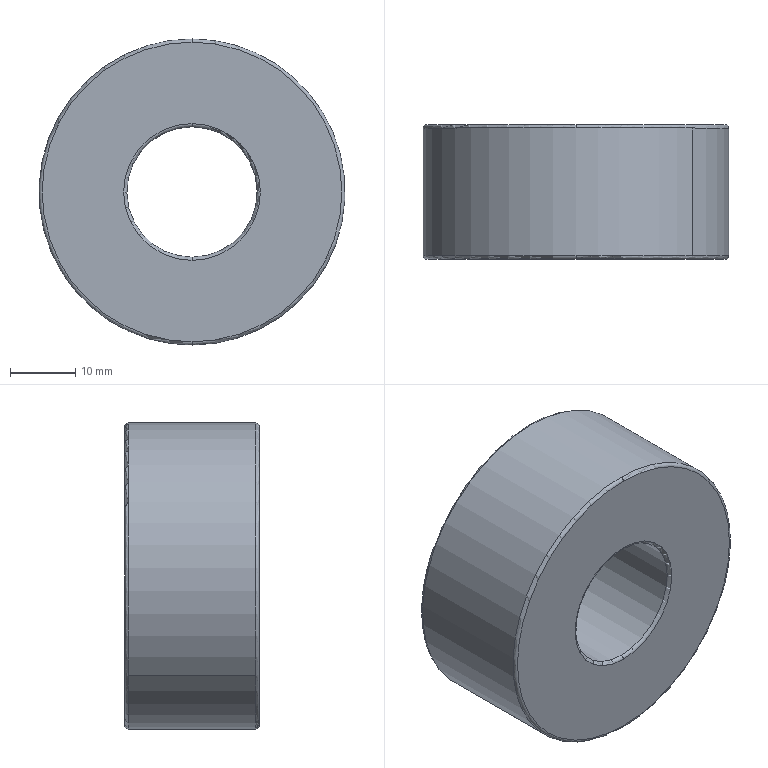Part | SolidWorks | features BaseBody 1 | 1 solid | 14 faces | box 47 x 20.6 x 47 mm | volume 29246 mm3 | torus 8 | cylinder 4 | plane 2 | commonest cylinder face diameters 20 x2 47 x2
STEP:
#1=CARTESIAN_POINT('',(624.451,36.7,7.283));
#2=VERTEX_POINT('',#1);
#3=CARTESIAN_POINT('',(624.451,36.7,28.283));
#4=VERTEX_POINT('',#3);
#5=CARTESIAN_POINT('',(624.451,36.7,17.783));
#6=DIRECTION('',(0.,1.,0.));
#7=DIRECTION('',(0.,0.,-1.));
#8=AXIS2_PLACEMENT_3D('',#5,#6,#7);
#9=CIRCLE('',#8,10.5);
#10=EDGE_CURVE('',#2,#4,#9,.T.);
#11=ORIENTED_EDGE('',*,*,#10,.F.);
#12=CARTESIAN_POINT('',(624.451,37.2,7.783));
#13=VERTEX_POINT('',#12);
#14=CARTESIAN_POINT('',(624.451,37.2,7.283));
#15=DIRECTION('',(-1.,0.,0.));
#16=DIRECTION('',(0.,0.,1.));
#17=AXIS2_PLACEMENT_3D('',#14,#15,#16);
#18=CIRCLE('',#17,0.5);
#19=EDGE_CURVE('',#2,#13,#18,.T.);
#20=ORIENTED_EDGE('',*,*,#19,.T.);
#21=CARTESIAN_POINT('',(616.859,37.2,11.275));
#22=VERTEX_POINT('',#21);
#23=CARTESIAN_POINT('',(624.451,37.2,17.783));
#24=DIRECTION('',(0.,1.,0.));
#25=DIRECTION('',(0.,0.,-1.));
#26=AXIS2_PLACEMENT_3D('',#23,#24,#25);
#27=CIRCLE('',#26,10.);
#28=EDGE_CURVE('',#13,#22,#27,.T.);
#29=ORIENTED_EDGE('',*,*,#28,.T.);
#30=CARTESIAN_POINT('',(624.451,37.2,27.783));
#31=VERTEX_POINT('',#30);
#32=CARTESIAN_POINT('',(624.451,37.2,17.783));
#33=DIRECTION('',(0.,1.,0.));
#34=DIRECTION('',(0.,0.,-1.));
#35=AXIS2_PLACEMENT_3D('',#32,#33,#34);
#36=CIRCLE('',#35,10.);
#37=EDGE_CURVE('',#22,#31,#36,.T.);
#38=ORIENTED_EDGE('',*,*,#37,.T.);
#39=CARTESIAN_POINT('',(624.451,37.2,28.283));
#40=DIRECTION('',(1.,0.,0.));
#41=DIRECTION('',(0.,0.,-1.));
#42=AXIS2_PLACEMENT_3D('',#39,#40,#41);
#43=CIRCLE('',#42,0.5);
#44=EDGE_CURVE('',#4,#31,#43,.T.);
#45=ORIENTED_EDGE('',*,*,#44,.F.);
#46=EDGE_LOOP('',(#11,#20,#29,#38,#45));
#47=FACE_OUTER_BOUND('',#46,.T.);
#48=CARTESIAN_POINT('',(624.451,37.2,17.783));
#49=DIRECTION('',(0.,-1.,0.));
#50=DIRECTION('',(0.,0.,1.));
#51=AXIS2_PLACEMENT_3D('',#48,#49,#50);
#52=TOROIDAL_SURFACE('',#51,10.5,0.5);
#53=ADVANCED_FACE('',(#47),#52,.T.);
#54=CARTESIAN_POINT('',(606.61,37.2,2.488));
#55=VERTEX_POINT('',#54);
#56=CARTESIAN_POINT('',(624.451,37.2,-5.717));
#57=VERTEX_POINT('',#56);
#58=CARTESIAN_POINT('',(624.451,37.2,17.783));
#59=DIRECTION('',(0.,-1.,0.));
#60=DIRECTION('',(0.,0.,-1.));
#61=AXIS2_PLACEMENT_3D('',#58,#59,#60);
#62=CIRCLE('',#61,23.5);
#63=EDGE_CURVE('',#55,#57,#62,.T.);
#64=ORIENTED_EDGE('',*,*,#63,.T.);
#65=CARTESIAN_POINT('',(624.451,36.7,-5.217));
#66=VERTEX_POINT('',#65);
#67=CARTESIAN_POINT('',(624.451,37.2,-5.217));
#68=DIRECTION('',(-1.,0.,0.));
#69=DIRECTION('',(0.,0.,1.));
#70=AXIS2_PLACEMENT_3D('',#67,#68,#69);
#71=CIRCLE('',#70,0.5);
#72=EDGE_CURVE('',#57,#66,#71,.T.);
#73=ORIENTED_EDGE('',*,*,#72,.T.);
#74=CARTESIAN_POINT('',(624.451,36.7,40.783));
#75=VERTEX_POINT('',#74);
#76=CARTESIAN_POINT('',(624.451,36.7,17.783));
#77=DIRECTION('',(0.,-1.,0.));
#78=DIRECTION('',(0.,0.,-1.));
#79=AXIS2_PLACEMENT_3D('',#76,#77,#78);
#80=CIRCLE('',#79,23.);
#81=EDGE_CURVE('',#75,#66,#80,.T.);
#82=ORIENTED_EDGE('',*,*,#81,.F.);
#83=CARTESIAN_POINT('',(624.451,37.2,41.283));
#84=VERTEX_POINT('',#83);
#85=CARTESIAN_POINT('',(624.451,37.2,40.783));
#86=DIRECTION('',(1.,0.,0.));
#87=DIRECTION('',(0.,0.,-1.));
#88=AXIS2_PLACEMENT_3D('',#85,#86,#87);
#89=CIRCLE('',#88,0.5);
#90=EDGE_CURVE('',#84,#75,#89,.T.);
#91=ORIENTED_EDGE('',*,*,#90,.F.);
#92=CARTESIAN_POINT('',(624.451,37.2,17.783));
#93=DIRECTION('',(0.,-1.,0.));
#94=DIRECTION('',(0.,0.,-1.));
#95=AXIS2_PLACEMENT_3D('',#92,#93,#94);
#96=CIRCLE('',#95,23.5);
#97=EDGE_CURVE('',#84,#55,#96,.T.);
#98=ORIENTED_EDGE('',*,*,#97,.T.);
#99=EDGE_LOOP('',(#64,#73,#82,#91,#98));
#100=FACE_OUTER_BOUND('',#99,.T.);
#101=CARTESIAN_POINT('',(624.451,37.2,17.783));
#102=DIRECTION('',(0.,-1.,0.));
#103=DIRECTION('',(0.,0.,1.));
#104=AXIS2_PLACEMENT_3D('',#101,#102,#103);
#105=TOROIDAL_SURFACE('',#104,23.,0.5);
#106=ADVANCED_FACE('',(#100),#105,.T.);
#107=CARTESIAN_POINT('',(624.451,56.8,41.283));
#108=VERTEX_POINT('',#107);
#109=CARTESIAN_POINT('',(606.61,56.8,2.488));
#110=VERTEX_POINT('',#109);
#111=CARTESIAN_POINT('',(624.451,56.8,17.783));
#112=DIRECTION('',(0.,-1.,0.));
#113=DIRECTION('',(0.,0.,1.));
#114=AXIS2_PLACEMENT_3D('',#111,#112,#113);
#115=CIRCLE('',#114,23.5);
#116=EDGE_CURVE('',#108,#110,#115,.T.);
#117=ORIENTED_EDGE('',*,*,#116,.F.);
#118=CARTESIAN_POINT('',(624.451,57.3,40.783));
#119=VERTEX_POINT('',#118);
#120=CARTESIAN_POINT('',(624.451,56.8,40.783));
#121=DIRECTION('',(-1.,0.,0.));
#122=DIRECTION('',(0.,0.,1.));
#123=AXIS2_PLACEMENT_3D('',#120,#121,#122);
#124=CIRCLE('',#123,0.5);
#125=EDGE_CURVE('',#108,#119,#124,.T.);
#126=ORIENTED_EDGE('',*,*,#125,.T.);
#127=CARTESIAN_POINT('',(624.451,57.3,-5.217));
#128=VERTEX_POINT('',#127);
#129=CARTESIAN_POINT('',(624.451,57.3,17.783));
#130=DIRECTION('',(0.,-1.,0.));
#131=DIRECTION('',(0.,0.,1.));
#132=AXIS2_PLACEMENT_3D('',#129,#130,#131);
#133=CIRCLE('',#132,23.);
#134=EDGE_CURVE('',#119,#128,#133,.T.);
#135=ORIENTED_EDGE('',*,*,#134,.T.);
#136=CARTESIAN_POINT('',(624.451,56.8,-5.717));
#137=VERTEX_POINT('',#136);
#138=CARTESIAN_POINT('',(624.451,56.8,-5.217));
#139=DIRECTION('',(1.,0.,0.));
#140=DIRECTION('',(0.,0.,-1.));
#141=AXIS2_PLACEMENT_3D('',#138,#139,#140);
#142=CIRCLE('',#141,0.5);
#143=EDGE_CURVE('',#137,#128,#142,.T.);
#144=ORIENTED_EDGE('',*,*,#143,.F.);
#145=CARTESIAN_POINT('',(624.451,56.8,17.783));
#146=DIRECTION('',(0.,-1.,0.));
#147=DIRECTION('',(0.,0.,1.));
#148=AXIS2_PLACEMENT_3D('',#145,#146,#147);
#149=CIRCLE('',#148,23.5);
#150=EDGE_CURVE('',#110,#137,#149,.T.);
#151=ORIENTED_EDGE('',*,*,#150,.F.);
#152=EDGE_LOOP('',(#117,#126,#135,#144,#151));
#153=FACE_OUTER_BOUND('',#152,.T.);
#154=CARTESIAN_POINT('',(624.451,56.8,17.783));
#155=DIRECTION('',(0.,1.,0.));
#156=DIRECTION('',(0.,0.,-1.));
#157=AXIS2_PLACEMENT_3D('',#154,#155,#156);
#158=TOROIDAL_SURFACE('',#157,23.,0.5);
#159=ADVANCED_FACE('',(#153),#158,.T.);
#160=CARTESIAN_POINT('',(624.451,57.3,7.283));
#161=VERTEX_POINT('',#160);
#162=CARTESIAN_POINT('',(624.451,57.3,28.283));
#163=VERTEX_POINT('',#162);
#164=CARTESIAN_POINT('',(624.451,57.3,17.783));
#165=DIRECTION('',(0.,1.,0.));
#166=DIRECTION('',(0.,0.,1.));
#167=AXIS2_PLACEMENT_3D('',#164,#165,#166);
#168=CIRCLE('',#167,10.5);
#169=EDGE_CURVE('',#161,#163,#168,.T.);
#170=ORIENTED_EDGE('',*,*,#169,.T.);
#171=CARTESIAN_POINT('',(624.451,56.8,27.783));
#172=VERTEX_POINT('',#171);
#173=CARTESIAN_POINT('',(624.451,56.8,28.283));
#174=DIRECTION('',(-1.,0.,0.));
#175=DIRECTION('',(0.,0.,1.));
#176=AXIS2_PLACEMENT_3D('',#173,#174,#175);
#177=CIRCLE('',#176,0.5);
#178=EDGE_CURVE('',#163,#172,#177,.T.);
#179=ORIENTED_EDGE('',*,*,#178,.T.);
#180=CARTESIAN_POINT('',(616.859,56.8,11.275));
#181=VERTEX_POINT('',#180);
#182=CARTESIAN_POINT('',(624.451,56.8,17.783));
#183=DIRECTION('',(0.,1.,0.));
#184=DIRECTION('',(0.,0.,1.));
#185=AXIS2_PLACEMENT_3D('',#182,#183,#184);
#186=CIRCLE('',#185,10.);
#187=EDGE_CURVE('',#181,#172,#186,.T.);
#188=ORIENTED_EDGE('',*,*,#187,.F.);
#189=CARTESIAN_POINT('',(624.451,56.8,7.783));
#190=VERTEX_POINT('',#189);
#191=CARTESIAN_POINT('',(624.451,56.8,17.783));
#192=DIRECTION('',(0.,1.,0.));
#193=DIRECTION('',(0.,0.,1.));
#194=AXIS2_PLACEMENT_3D('',#191,#192,#193);
#195=CIRCLE('',#194,10.);
#196=EDGE_CURVE('',#190,#181,#195,.T.);
#197=ORIENTED_EDGE('',*,*,#196,.F.);
#198=CARTESIAN_POINT('',(624.451,56.8,7.283));
#199=DIRECTION('',(1.,0.,0.));
#200=DIRECTION('',(0.,0.,-1.));
#201=AXIS2_PLACEMENT_3D('',#198,#199,#200);
#202=CIRCLE('',#201,0.5);
#203=EDGE_CURVE('',#161,#190,#202,.T.);
#204=ORIENTED_EDGE('',*,*,#203,.F.);
#205=EDGE_LOOP('',(#170,#179,#188,#197,#204));
#206=FACE_OUTER_BOUND('',#205,.T.);
#207=CARTESIAN_POINT('',(624.451,56.8,17.783));
#208=DIRECTION('',(0.,1.,0.));
#209=DIRECTION('',(0.,0.,-1.));
#210=AXIS2_PLACEMENT_3D('',#207,#208,#209);
#211=TOROIDAL_SURFACE('',#210,10.5,0.5);
#212=ADVANCED_FACE('',(#206),#211,.T.);
#213=ORIENTED_EDGE('',*,*,#187,.T.);
#214=CARTESIAN_POINT('',(632.043,56.8,24.292));
#215=VERTEX_POINT('',#214);
#216=CARTESIAN_POINT('',(624.451,56.8,17.783));
#217=DIRECTION('',(0.,1.,0.));
#218=DIRECTION('',(0.,0.,1.));
#219=AXIS2_PLACEMENT_3D('',#216,#217,#218);
#220=CIRCLE('',#219,10.);
#221=EDGE_CURVE('',#172,#215,#220,.T.);
#222=ORIENTED_EDGE('',*,*,#221,.T.);
#223=CARTESIAN_POINT('',(632.043,37.2,24.292));
#224=VERTEX_POINT('',#223);
#225=CARTESIAN_POINT('',(632.043,46.7,24.292));
#226=DIRECTION('',(0.,-1.,0.));
#227=VECTOR('',#226,1000.);
#228=LINE('',#225,#227);
#229=EDGE_CURVE('',#215,#224,#228,.T.);
#230=ORIENTED_EDGE('',*,*,#229,.T.);
#231=CARTESIAN_POINT('',(624.451,37.2,17.783));
#232=DIRECTION('',(0.,1.,0.));
#233=DIRECTION('',(0.,0.,-1.));
#234=AXIS2_PLACEMENT_3D('',#231,#232,#233);
#235=CIRCLE('',#234,10.);
#236=EDGE_CURVE('',#31,#224,#235,.T.);
#237=ORIENTED_EDGE('',*,*,#236,.F.);
#238=ORIENTED_EDGE('',*,*,#37,.F.);
#239=CARTESIAN_POINT('',(616.859,46.7,11.275));
#240=DIRECTION('',(0.,-1.,0.));
#241=VECTOR('',#240,1000.);
#242=LINE('',#239,#241);
#243=EDGE_CURVE('',#181,#22,#242,.T.);
#244=ORIENTED_EDGE('',*,*,#243,.F.);
#245=EDGE_LOOP('',(#213,#222,#230,#237,#238,#244));
#246=FACE_OUTER_BOUND('',#245,.T.);
#247=CARTESIAN_POINT('',(624.451,46.7,17.783));
#248=DIRECTION('',(0.,-1.,0.));
#249=DIRECTION('',(-0.7592,0.,-0.6509));
#250=AXIS2_PLACEMENT_3D('',#247,#248,#249);
#251=CYLINDRICAL_SURFACE('',#250,10.);
#252=ADVANCED_FACE('',(#246),#251,.F.);
#253=ORIENTED_EDGE('',*,*,#150,.T.);
#254=CARTESIAN_POINT('',(642.292,56.8,33.079));
#255=VERTEX_POINT('',#254);
#256=CARTESIAN_POINT('',(624.451,56.8,17.783));
#257=DIRECTION('',(0.,-1.,0.));
#258=DIRECTION('',(0.,0.,1.));
#259=AXIS2_PLACEMENT_3D('',#256,#257,#258);
#260=CIRCLE('',#259,23.5);
#261=EDGE_CURVE('',#137,#255,#260,.T.);
#262=ORIENTED_EDGE('',*,*,#261,.T.);
#263=CARTESIAN_POINT('',(642.292,37.2,33.079));
#264=VERTEX_POINT('',#263);
#265=CARTESIAN_POINT('',(642.292,46.7,33.079));
#266=DIRECTION('',(0.,-1.,0.));
#267=VECTOR('',#266,1000.);
#268=LINE('',#265,#267);
#269=EDGE_CURVE('',#255,#264,#268,.T.);
#270=ORIENTED_EDGE('',*,*,#269,.T.);
#271=CARTESIAN_POINT('',(624.451,37.2,17.783));
#272=DIRECTION('',(0.,-1.,0.));
#273=DIRECTION('',(0.,0.,-1.));
#274=AXIS2_PLACEMENT_3D('',#271,#272,#273);
#275=CIRCLE('',#274,23.5);
#276=EDGE_CURVE('',#57,#264,#275,.T.);
#277=ORIENTED_EDGE('',*,*,#276,.F.);
#278=ORIENTED_EDGE('',*,*,#63,.F.);
#279=CARTESIAN_POINT('',(606.61,46.7,2.488));
#280=DIRECTION('',(0.,-1.,0.));
#281=VECTOR('',#280,1000.);
#282=LINE('',#279,#281);
#283=EDGE_CURVE('',#110,#55,#282,.T.);
#284=ORIENTED_EDGE('',*,*,#283,.F.);
#285=EDGE_LOOP('',(#253,#262,#270,#277,#278,#284));
#286=FACE_OUTER_BOUND('',#285,.T.);
#287=CARTESIAN_POINT('',(624.451,46.7,17.783));
#288=DIRECTION('',(0.,-1.,0.));
#289=DIRECTION('',(-0.7592,0.,-0.6509));
#290=AXIS2_PLACEMENT_3D('',#287,#288,#289);
#291=CYLINDRICAL_SURFACE('',#290,23.5);
#292=ADVANCED_FACE('',(#286),#291,.T.);
#293=CARTESIAN_POINT('',(624.451,36.7,17.783));
#294=DIRECTION('',(0.,1.,0.));
#295=DIRECTION('',(0.,0.,-1.));
#296=AXIS2_PLACEMENT_3D('',#293,#294,#295);
#297=CIRCLE('',#296,10.5);
#298=EDGE_CURVE('',#4,#2,#297,.T.);
#299=ORIENTED_EDGE('',*,*,#298,.T.);
#300=ORIENTED_EDGE('',*,*,#10,.T.);
#301=EDGE_LOOP('',(#299,#300));
#302=FACE_BOUND('',#301,.T.);
#303=ORIENTED_EDGE('',*,*,#81,.T.);
#304=CARTESIAN_POINT('',(624.451,36.7,17.783));
#305=DIRECTION('',(0.,-1.,0.));
#306=DIRECTION('',(0.,0.,-1.));
#307=AXIS2_PLACEMENT_3D('',#304,#305,#306);
#308=CIRCLE('',#307,23.);
#309=EDGE_CURVE('',#66,#75,#308,.T.);
#310=ORIENTED_EDGE('',*,*,#309,.T.);
#311=EDGE_LOOP('',(#303,#310));
#312=FACE_OUTER_BOUND('',#311,.T.);
#313=CARTESIAN_POINT('',(624.451,36.7,17.783));
#314=DIRECTION('',(0.,-1.,0.));
#315=DIRECTION('',(0.,0.,-1.));
#316=AXIS2_PLACEMENT_3D('',#313,#314,#315);
#317=PLANE('',#316);
#318=ADVANCED_FACE('',(#302,#312),#317,.T.);
#319=ORIENTED_EDGE('',*,*,#269,.F.);
#320=CARTESIAN_POINT('',(624.451,56.8,17.783));
#321=DIRECTION('',(0.,-1.,0.));
#322=DIRECTION('',(0.,0.,1.));
#323=AXIS2_PLACEMENT_3D('',#320,#321,#322);
#324=CIRCLE('',#323,23.5);
#325=EDGE_CURVE('',#255,#108,#324,.T.);
#326=ORIENTED_EDGE('',*,*,#325,.T.);
#327=ORIENTED_EDGE('',*,*,#116,.T.);
#328=ORIENTED_EDGE('',*,*,#283,.T.);
#329=ORIENTED_EDGE('',*,*,#97,.F.);
#330=CARTESIAN_POINT('',(624.451,37.2,17.783));
#331=DIRECTION('',(0.,-1.,0.));
#332=DIRECTION('',(0.,0.,-1.));
#333=AXIS2_PLACEMENT_3D('',#330,#331,#332);
#334=CIRCLE('',#333,23.5);
#335=EDGE_CURVE('',#264,#84,#334,.T.);
#336=ORIENTED_EDGE('',*,*,#335,.F.);
#337=EDGE_LOOP('',(#319,#326,#327,#328,#329,#336));
#338=FACE_OUTER_BOUND('',#337,.T.);
#339=CARTESIAN_POINT('',(624.451,46.7,17.783));
#340=DIRECTION('',(0.,-1.,0.));
#341=DIRECTION('',(-0.7592,0.,-0.6509));
#342=AXIS2_PLACEMENT_3D('',#339,#340,#341);
#343=CYLINDRICAL_SURFACE('',#342,23.5);
#344=ADVANCED_FACE('',(#338),#343,.T.);
#345=ORIENTED_EDGE('',*,*,#169,.F.);
#346=CARTESIAN_POINT('',(624.451,57.3,17.783));
#347=DIRECTION('',(0.,1.,0.));
#348=DIRECTION('',(0.,0.,1.));
#349=AXIS2_PLACEMENT_3D('',#346,#347,#348);
#350=CIRCLE('',#349,10.5);
#351=EDGE_CURVE('',#163,#161,#350,.T.);
#352=ORIENTED_EDGE('',*,*,#351,.F.);
#353=EDGE_LOOP('',(#345,#352));
#354=FACE_BOUND('',#353,.T.);
#355=CARTESIAN_POINT('',(624.451,57.3,17.783));
#356=DIRECTION('',(0.,-1.,0.));
#357=DIRECTION('',(0.,0.,1.));
#358=AXIS2_PLACEMENT_3D('',#355,#356,#357);
#359=CIRCLE('',#358,23.);
#360=EDGE_CURVE('',#128,#119,#359,.T.);
#361=ORIENTED_EDGE('',*,*,#360,.F.);
#362=ORIENTED_EDGE('',*,*,#134,.F.);
#363=EDGE_LOOP('',(#361,#362));
#364=FACE_OUTER_BOUND('',#363,.T.);
#365=CARTESIAN_POINT('',(624.451,57.3,17.783));
#366=DIRECTION('',(0.,1.,0.));
#367=DIRECTION('',(1.,0.,0.));
#368=AXIS2_PLACEMENT_3D('',#365,#366,#367);
#369=PLANE('',#368);
#370=ADVANCED_FACE('',(#354,#364),#369,.T.);
#371=ORIENTED_EDGE('',*,*,#229,.F.);
#372=CARTESIAN_POINT('',(624.451,56.8,17.783));
#373=DIRECTION('',(0.,1.,0.));
#374=DIRECTION('',(0.,0.,1.));
#375=AXIS2_PLACEMENT_3D('',#372,#373,#374);
#376=CIRCLE('',#375,10.);
#377=EDGE_CURVE('',#215,#190,#376,.T.);
#378=ORIENTED_EDGE('',*,*,#377,.T.);
#379=ORIENTED_EDGE('',*,*,#196,.T.);
#380=ORIENTED_EDGE('',*,*,#243,.T.);
#381=ORIENTED_EDGE('',*,*,#28,.F.);
#382=CARTESIAN_POINT('',(624.451,37.2,17.783));
#383=DIRECTION('',(0.,1.,0.));
#384=DIRECTION('',(0.,0.,-1.));
#385=AXIS2_PLACEMENT_3D('',#382,#383,#384);
#386=CIRCLE('',#385,10.);
#387=EDGE_CURVE('',#224,#13,#386,.T.);
#388=ORIENTED_EDGE('',*,*,#387,.F.);
#389=EDGE_LOOP('',(#371,#378,#379,#380,#381,#388));
#390=FACE_OUTER_BOUND('',#389,.T.);
#391=CARTESIAN_POINT('',(624.451,46.7,17.783));
#392=DIRECTION('',(0.,-1.,0.));
#393=DIRECTION('',(-0.7592,0.,-0.6509));
#394=AXIS2_PLACEMENT_3D('',#391,#392,#393);
#395=CYLINDRICAL_SURFACE('',#394,10.);
#396=ADVANCED_FACE('',(#390),#395,.F.);
#397=ORIENTED_EDGE('',*,*,#178,.F.);
#398=ORIENTED_EDGE('',*,*,#351,.T.);
#399=ORIENTED_EDGE('',*,*,#203,.T.);
#400=ORIENTED_EDGE('',*,*,#377,.F.);
#401=ORIENTED_EDGE('',*,*,#221,.F.);
#402=EDGE_LOOP('',(#397,#398,#399,#400,#401));
#403=FACE_OUTER_BOUND('',#402,.T.);
#404=CARTESIAN_POINT('',(624.451,56.8,17.783));
#405=DIRECTION('',(0.,1.,0.));
#406=DIRECTION('',(0.,0.,-1.));
#407=AXIS2_PLACEMENT_3D('',#404,#405,#406);
#408=TOROIDAL_SURFACE('',#407,10.5,0.5);
#409=ADVANCED_FACE('',(#403),#408,.T.);
#410=ORIENTED_EDGE('',*,*,#125,.F.);
#411=ORIENTED_EDGE('',*,*,#325,.F.);
#412=ORIENTED_EDGE('',*,*,#261,.F.);
#413=ORIENTED_EDGE('',*,*,#143,.T.);
#414=ORIENTED_EDGE('',*,*,#360,.T.);
#415=EDGE_LOOP('',(#410,#411,#412,#413,#414));
#416=FACE_OUTER_BOUND('',#415,.T.);
#417=CARTESIAN_POINT('',(624.451,56.8,17.783));
#418=DIRECTION('',(0.,1.,0.));
#419=DIRECTION('',(0.,0.,-1.));
#420=AXIS2_PLACEMENT_3D('',#417,#418,#419);
#421=TOROIDAL_SURFACE('',#420,23.,0.5);
#422=ADVANCED_FACE('',(#416),#421,.T.);
#423=ORIENTED_EDGE('',*,*,#72,.F.);
#424=ORIENTED_EDGE('',*,*,#276,.T.);
#425=ORIENTED_EDGE('',*,*,#335,.T.);
#426=ORIENTED_EDGE('',*,*,#90,.T.);
#427=ORIENTED_EDGE('',*,*,#309,.F.);
#428=EDGE_LOOP('',(#423,#424,#425,#426,#427));
#429=FACE_OUTER_BOUND('',#428,.T.);
#430=CARTESIAN_POINT('',(624.451,37.2,17.783));
#431=DIRECTION('',(0.,-1.,0.));
#432=DIRECTION('',(0.,0.,1.));
#433=AXIS2_PLACEMENT_3D('',#430,#431,#432);
#434=TOROIDAL_SURFACE('',#433,23.,0.5);
#435=ADVANCED_FACE('',(#429),#434,.T.);
#436=ORIENTED_EDGE('',*,*,#19,.F.);
#437=ORIENTED_EDGE('',*,*,#298,.F.);
#438=ORIENTED_EDGE('',*,*,#44,.T.);
#439=ORIENTED_EDGE('',*,*,#236,.T.);
#440=ORIENTED_EDGE('',*,*,#387,.T.);
#441=EDGE_LOOP('',(#436,#437,#438,#439,#440));
#442=FACE_OUTER_BOUND('',#441,.T.);
#443=CARTESIAN_POINT('',(624.451,37.2,17.783));
#444=DIRECTION('',(0.,-1.,0.));
#445=DIRECTION('',(0.,0.,1.));
#446=AXIS2_PLACEMENT_3D('',#443,#444,#445);
#447=TOROIDAL_SURFACE('',#446,10.5,0.5);
#448=ADVANCED_FACE('',(#442),#447,.T.);
#449=CLOSED_SHELL('',(#53,#106,#159,#212,#252,#292,#318,#344,#370,#396,#409,#422,#435,#448));
#450=MANIFOLD_SOLID_BREP('',#449);
#451=CARTESIAN_POINT('',(0.,0.,0.));
#452=DIRECTION('',(0.,0.,1.));
#453=DIRECTION('',(1.,0.,0.));
#454=AXIS2_PLACEMENT_3D('',#451,#452,#453);
#455=(LENGTH_UNIT()NAMED_UNIT(*)SI_UNIT(.MILLI.,.METRE.));
#456=UNCERTAINTY_MEASURE_WITH_UNIT(LENGTH_MEASURE(0.00001),#455,'','');
#457=(NAMED_UNIT(*)PLANE_ANGLE_UNIT()SI_UNIT($,.RADIAN.));
#458=(NAMED_UNIT(*)SI_UNIT($,.STERADIAN.)SOLID_ANGLE_UNIT());
#459=(GEOMETRIC_REPRESENTATION_CONTEXT(3)GLOBAL_UNCERTAINTY_ASSIGNED_CONTEXT((#456))GLOBAL_UNIT_ASSIGNED_CONTEXT((#455,#457,#458))REPRESENTATION_CONTEXT('',''));
#460=ADVANCED_BREP_SHAPE_REPRESENTATION('',(#450,#454),#459);